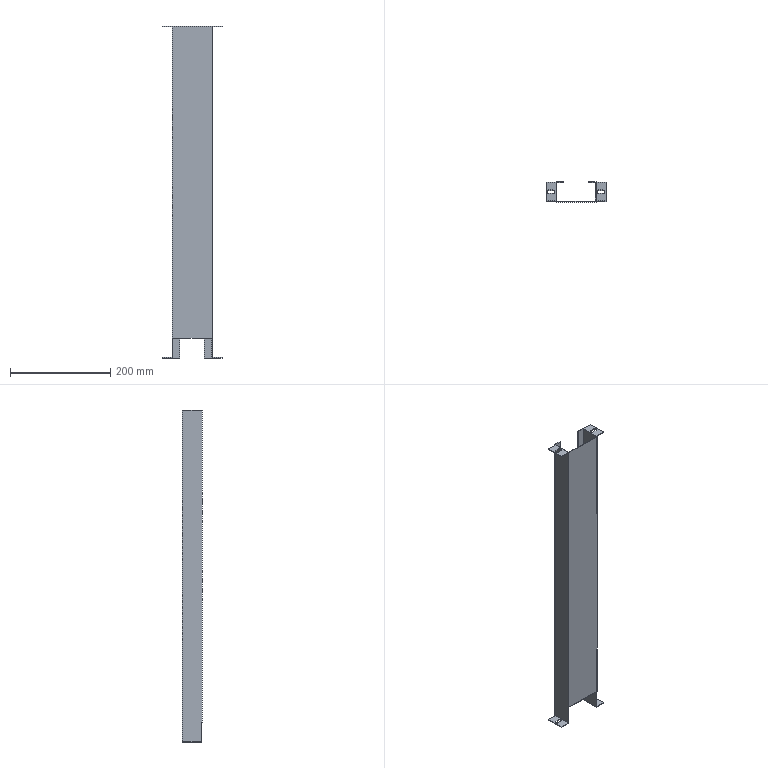Part | STEP file | 1 solid | 56 faces | box 120 x 40 x 664 mm | volume 146043 mm3 | plane 40 | cylinder 16 | commonest cylinder face diameters 7 x12 20 x4